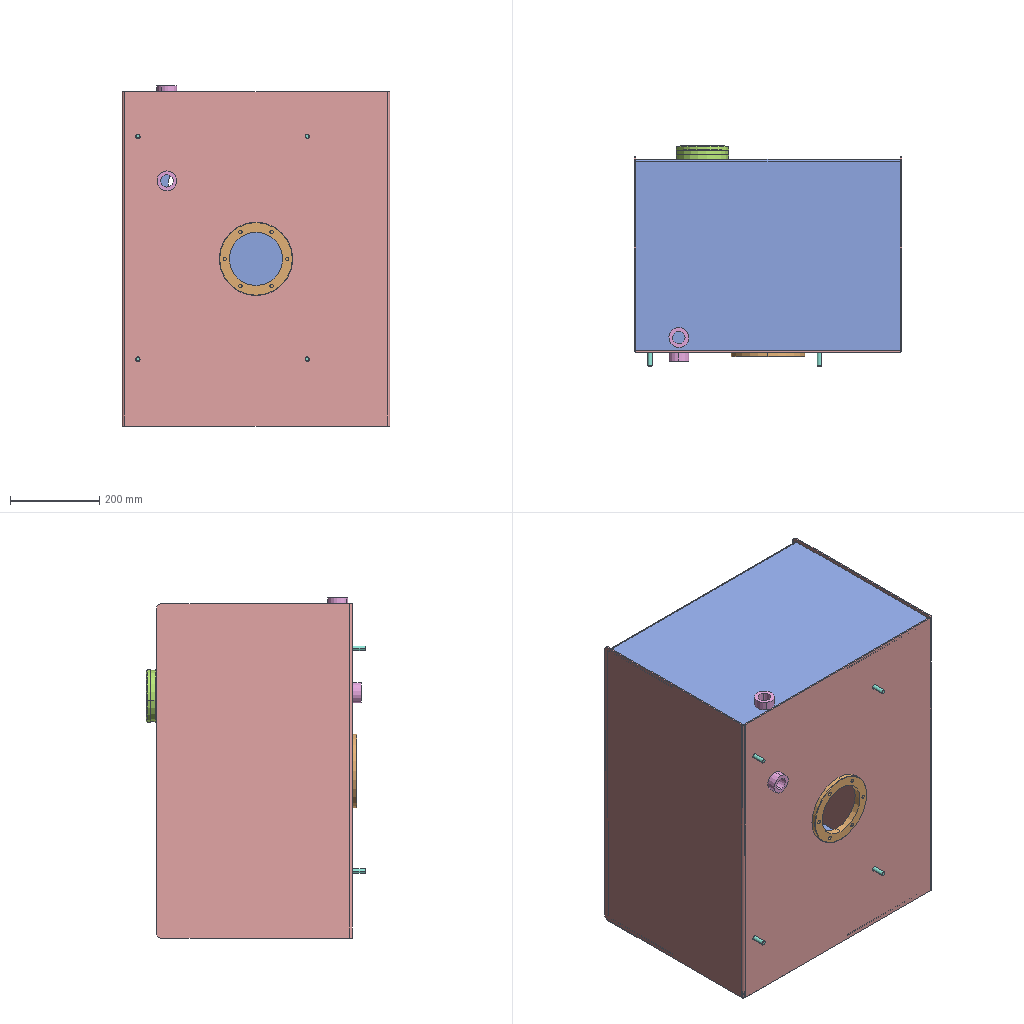Assembly | SolidWorks | 6 different items | 10 placed | box 600 x 493 x 763 mm
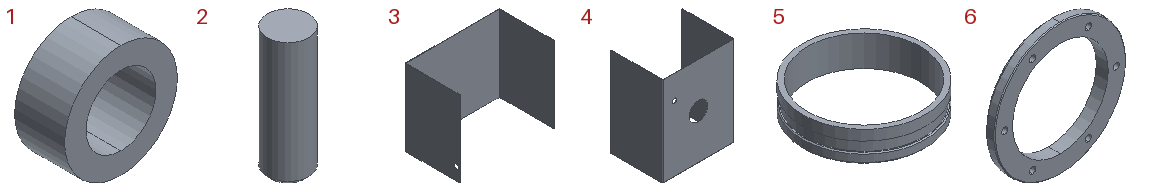Parts list (item | quantity | size | volume | features):
1 | x2 | 45 x 23 x 45 mm | 20479 mm3 | features Chamfer 1, Extrusion 1, ICE 1
2 | x4 | 10 x 10 x 30 mm | 2342 mm3 | features Chamfer 1, Extrusion 1
3 | x1 | 736 x 430 x 594 mm | 2800017 mm3 | features ICE 3, FlatPattern 1, SMBaseFlange 1, SheetMetal 1
4 | x1 | 600 x 440 x 750 mm | 3247324 mm3 | features ICE 2, FlatPattern 1, SMBaseFlange 1, SheetMetal 1
5 | x1 | 120 x 120 x 30 mm | 45845 mm3 | features Chamfer 2, ICE 2, Extrusion 1
6 | x1 | 165 x 15 x 165 mm | 136377 mm3 | features Chamfer 2, ICE 2, Extrusion 1
Mates (type | each side: item.copy, entity, surface, feature):
Coincident | 4.1 face plane Base-Flange1 | 3.1 face plane Base-Flange1 | 2 times
DistanceDim | 3.1 face plane Base-Flange1 | 4.1 face plane Base-Flange1
Concentric | 3.1 edge | 5.1 edge
Coincident | 3.1 face plane Base-Flange1 | 5.1 face plane Boss-Extrude2
Concentric | 4.1 edge | 1.1 edge
Coincident | 4.1 face plane Base-Flange1 | 1.1 face plane Cut-Extrude1
Concentric | 3.1 edge | 1.2 edge
Coincident | 3.1 face plane Base-Flange1 | 1.2 face plane Cut-Extrude1
Coincident | 4.1 face plane Base-Flange1 | 2.1 face plane Boss-Extrude1
Concentric | 2.1 edge | assembly select_type:10
Coincident | 2.1 face plane Boss-Extrude1 | 2.2 face plane Boss-Extrude1
Coincident | 4.1 face plane Base-Flange1 | assembly face
Coincident | 2.2 face plane Boss-Extrude1 | 2.3 face plane Boss-Extrude1
Coincident | 2.2 face plane Boss-Extrude1 | 2.4 face plane Boss-Extrude1
Concentric | 2.3 edge | assembly select_type:10
Concentric | 2.4 edge | assembly select_type:10
Concentric | 2.2 edge | assembly select_type:10
Coincident | 4.1 face plane Base-Flange1 | 6.1 face plane Cut-Extrude1
Concentric | 4.1 edge | 6.1 edge